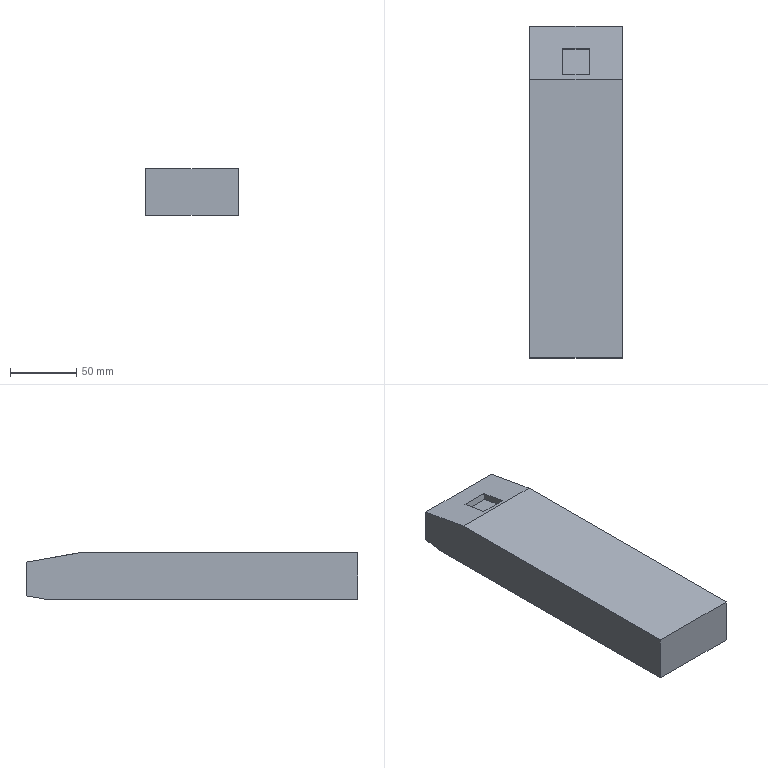Part | STEP file | 1 solid | 13 faces | box 70 x 250 x 35 mm | volume 599290 mm3 | plane 13
STEP:
#1=CARTESIAN_POINT('',(0.,0.,0.));
#2=DIRECTION('',(0.,0.,1.));
#3=DIRECTION('',(1.,0.,0.));
#4=AXIS2_PLACEMENT_3D('',#1,#2,#3);
#5=CARTESIAN_POINT('',(-77.862,-165.,-78.92));
#6=VERTEX_POINT('',#5);
#7=CARTESIAN_POINT('',(-77.862,-165.,-113.92));
#8=VERTEX_POINT('',#7);
#9=CARTESIAN_POINT('',(-77.862,-165.,-78.92));
#10=DIRECTION('',(0.,0.,-1.));
#11=VECTOR('',#10,1.);
#12=LINE('',#9,#11);
#13=CARTESIAN_POINT('',(-77.862,-165.,-113.92));
#14=DIRECTION('',(0.,-1.,0.));
#15=DIRECTION('',(0.,0.,-1.));
#16=AXIS2_PLACEMENT_3D('',#13,#14,#15);
#17=PLANE('',#16);
#18=CARTESIAN_POINT('',(-35.,0.));
#19=DIRECTION('',(1.,0.));
#20=VECTOR('',#19,1.);
#21=LINE('',#18,#20);
#22=(GEOMETRIC_REPRESENTATION_CONTEXT(2)PARAMETRIC_REPRESENTATION_CONTEXT()REPRESENTATION_CONTEXT('',''));
#23=DEFINITIONAL_REPRESENTATION('',(#21),#22);
#24=PCURVE('',#17,#23);
#25=CARTESIAN_POINT('',(-77.862,-150.,-78.92));
#26=DIRECTION('',(1.,0.,0.));
#27=DIRECTION('',(0.,0.,-1.));
#28=AXIS2_PLACEMENT_3D('',#25,#26,#27);
#29=PLANE('',#28);
#30=CARTESIAN_POINT('',(0.,-15.));
#31=DIRECTION('',(1.,0.));
#32=VECTOR('',#31,1.);
#33=LINE('',#30,#32);
#34=(GEOMETRIC_REPRESENTATION_CONTEXT(2)PARAMETRIC_REPRESENTATION_CONTEXT()REPRESENTATION_CONTEXT('',''));
#35=DEFINITIONAL_REPRESENTATION('',(#33),#34);
#36=PCURVE('',#29,#35);
#37=SURFACE_CURVE('',#12,(#24,#36),.PCURVE_S1.);
#38=EDGE_CURVE('',#6,#8,#37,.T.);
#39=ORIENTED_EDGE('',*,*,#38,.T.);
#40=CARTESIAN_POINT('',(-7.863,-165.,-113.92));
#41=VERTEX_POINT('',#40);
#42=CARTESIAN_POINT('',(-77.862,-165.,-113.92));
#43=DIRECTION('',(1.,0.,0.));
#44=VECTOR('',#43,1.);
#45=LINE('',#42,#44);
#46=CARTESIAN_POINT('',(0.,0.));
#47=DIRECTION('',(0.,1.));
#48=VECTOR('',#47,1.);
#49=LINE('',#46,#48);
#50=(GEOMETRIC_REPRESENTATION_CONTEXT(2)PARAMETRIC_REPRESENTATION_CONTEXT()REPRESENTATION_CONTEXT('',''));
#51=DEFINITIONAL_REPRESENTATION('',(#49),#50);
#52=PCURVE('',#17,#51);
#53=CARTESIAN_POINT('',(-77.862,-150.,-113.92));
#54=DIRECTION('',(0.,0.,1.));
#55=DIRECTION('',(1.,0.,0.));
#56=AXIS2_PLACEMENT_3D('',#53,#54,#55);
#57=PLANE('',#56);
#58=CARTESIAN_POINT('',(0.,-15.));
#59=DIRECTION('',(1.,0.));
#60=VECTOR('',#59,1.);
#61=LINE('',#58,#60);
#62=(GEOMETRIC_REPRESENTATION_CONTEXT(2)PARAMETRIC_REPRESENTATION_CONTEXT()REPRESENTATION_CONTEXT('',''));
#63=DEFINITIONAL_REPRESENTATION('',(#61),#62);
#64=PCURVE('',#57,#63);
#65=SURFACE_CURVE('',#45,(#52,#64),.PCURVE_S1.);
#66=EDGE_CURVE('',#8,#41,#65,.T.);
#67=ORIENTED_EDGE('',*,*,#66,.T.);
#68=CARTESIAN_POINT('',(-7.863,-165.,-78.92));
#69=VERTEX_POINT('',#68);
#70=CARTESIAN_POINT('',(-7.863,-165.,-113.92));
#71=DIRECTION('',(0.,0.,1.));
#72=VECTOR('',#71,1.);
#73=LINE('',#70,#72);
#74=CARTESIAN_POINT('',(0.,70.));
#75=DIRECTION('',(-1.,0.));
#76=VECTOR('',#75,1.);
#77=LINE('',#74,#76);
#78=(GEOMETRIC_REPRESENTATION_CONTEXT(2)PARAMETRIC_REPRESENTATION_CONTEXT()REPRESENTATION_CONTEXT('',''));
#79=DEFINITIONAL_REPRESENTATION('',(#77),#78);
#80=PCURVE('',#17,#79);
#81=CARTESIAN_POINT('',(-7.863,-150.,-113.92));
#82=DIRECTION('',(-1.,0.,0.));
#83=DIRECTION('',(0.,0.,1.));
#84=AXIS2_PLACEMENT_3D('',#81,#82,#83);
#85=PLANE('',#84);
#86=CARTESIAN_POINT('',(0.,-15.));
#87=DIRECTION('',(1.,0.));
#88=VECTOR('',#87,1.);
#89=LINE('',#86,#88);
#90=(GEOMETRIC_REPRESENTATION_CONTEXT(2)PARAMETRIC_REPRESENTATION_CONTEXT()REPRESENTATION_CONTEXT('',''));
#91=DEFINITIONAL_REPRESENTATION('',(#89),#90);
#92=PCURVE('',#85,#91);
#93=SURFACE_CURVE('',#73,(#80,#92),.PCURVE_S1.);
#94=EDGE_CURVE('',#41,#69,#93,.T.);
#95=ORIENTED_EDGE('',*,*,#94,.T.);
#96=CARTESIAN_POINT('',(-7.863,-165.,-78.92));
#97=DIRECTION('',(-1.,0.,0.));
#98=VECTOR('',#97,1.);
#99=LINE('',#96,#98);
#100=CARTESIAN_POINT('',(-35.,70.));
#101=DIRECTION('',(0.,-1.));
#102=VECTOR('',#101,1.);
#103=LINE('',#100,#102);
#104=(GEOMETRIC_REPRESENTATION_CONTEXT(2)PARAMETRIC_REPRESENTATION_CONTEXT()REPRESENTATION_CONTEXT('',''));
#105=DEFINITIONAL_REPRESENTATION('',(#103),#104);
#106=PCURVE('',#17,#105);
#107=CARTESIAN_POINT('',(-7.863,-150.,-78.92));
#108=DIRECTION('',(0.,0.,-1.));
#109=DIRECTION('',(-1.,0.,0.));
#110=AXIS2_PLACEMENT_3D('',#107,#108,#109);
#111=PLANE('',#110);
#112=CARTESIAN_POINT('',(0.,-15.));
#113=DIRECTION('',(1.,0.));
#114=VECTOR('',#113,1.);
#115=LINE('',#112,#114);
#116=(GEOMETRIC_REPRESENTATION_CONTEXT(2)PARAMETRIC_REPRESENTATION_CONTEXT()REPRESENTATION_CONTEXT('',''));
#117=DEFINITIONAL_REPRESENTATION('',(#115),#116);
#118=PCURVE('',#111,#117);
#119=SURFACE_CURVE('',#99,(#106,#118),.PCURVE_S1.);
#120=EDGE_CURVE('',#69,#6,#119,.T.);
#121=ORIENTED_EDGE('',*,*,#120,.T.);
#122=EDGE_LOOP('',(#39,#67,#95,#121));
#123=FACE_BOUND('',#122,.T.);
#124=ADVANCED_FACE('',(#123),#17,.T.);
#125=CARTESIAN_POINT('',(-7.863,45.,-78.92));
#126=VERTEX_POINT('',#125);
#127=CARTESIAN_POINT('',(-7.863,-150.,-78.92));
#128=DIRECTION('',(0.,1.,0.));
#129=VECTOR('',#128,1.);
#130=LINE('',#127,#129);
#131=CARTESIAN_POINT('',(0.,0.));
#132=DIRECTION('',(0.,1.));
#133=VECTOR('',#132,1.);
#134=LINE('',#131,#133);
#135=(GEOMETRIC_REPRESENTATION_CONTEXT(2)PARAMETRIC_REPRESENTATION_CONTEXT()REPRESENTATION_CONTEXT('',''));
#136=DEFINITIONAL_REPRESENTATION('',(#134),#135);
#137=PCURVE('',#111,#136);
#138=CARTESIAN_POINT('',(35.,0.));
#139=DIRECTION('',(0.,1.));
#140=VECTOR('',#139,1.);
#141=LINE('',#138,#140);
#142=(GEOMETRIC_REPRESENTATION_CONTEXT(2)PARAMETRIC_REPRESENTATION_CONTEXT()REPRESENTATION_CONTEXT('',''));
#143=DEFINITIONAL_REPRESENTATION('',(#141),#142);
#144=PCURVE('',#85,#143);
#145=SURFACE_CURVE('',#130,(#137,#144),.PCURVE_S1.);
#146=EDGE_CURVE('',#69,#126,#145,.T.);
#147=ORIENTED_EDGE('',*,*,#146,.T.);
#148=CARTESIAN_POINT('',(-77.862,45.,-78.92));
#149=VERTEX_POINT('',#148);
#150=CARTESIAN_POINT('',(-7.863,45.,-78.92));
#151=DIRECTION('',(-1.,0.,0.));
#152=VECTOR('',#151,1.);
#153=LINE('',#150,#152);
#154=CARTESIAN_POINT('',(0.,195.));
#155=DIRECTION('',(1.,0.));
#156=VECTOR('',#155,1.);
#157=LINE('',#154,#156);
#158=(GEOMETRIC_REPRESENTATION_CONTEXT(2)PARAMETRIC_REPRESENTATION_CONTEXT()REPRESENTATION_CONTEXT('',''));
#159=DEFINITIONAL_REPRESENTATION('',(#157),#158);
#160=PCURVE('',#111,#159);
#161=CARTESIAN_POINT('',(-7.863,45.,-78.92));
#162=DIRECTION('',(0.,0.1736,0.9848));
#163=DIRECTION('',(0.,-0.9848,0.1736));
#164=AXIS2_PLACEMENT_3D('',#161,#162,#163);
#165=PLANE('',#164);
#166=CARTESIAN_POINT('',(0.,0.));
#167=DIRECTION('',(0.,-1.));
#168=VECTOR('',#167,1.);
#169=LINE('',#166,#168);
#170=(GEOMETRIC_REPRESENTATION_CONTEXT(2)PARAMETRIC_REPRESENTATION_CONTEXT()REPRESENTATION_CONTEXT('',''));
#171=DEFINITIONAL_REPRESENTATION('',(#169),#170);
#172=PCURVE('',#165,#171);
#173=SURFACE_CURVE('',#153,(#160,#172),.PCURVE_S1.);
#174=EDGE_CURVE('',#126,#149,#173,.T.);
#175=ORIENTED_EDGE('',*,*,#174,.T.);
#176=CARTESIAN_POINT('',(-77.862,-150.,-78.92));
#177=DIRECTION('',(0.,1.,0.));
#178=VECTOR('',#177,1.);
#179=LINE('',#176,#178);
#180=CARTESIAN_POINT('',(70.,0.));
#181=DIRECTION('',(0.,1.));
#182=VECTOR('',#181,1.);
#183=LINE('',#180,#182);
#184=(GEOMETRIC_REPRESENTATION_CONTEXT(2)PARAMETRIC_REPRESENTATION_CONTEXT()REPRESENTATION_CONTEXT('',''));
#185=DEFINITIONAL_REPRESENTATION('',(#183),#184);
#186=PCURVE('',#111,#185);
#187=CARTESIAN_POINT('',(0.,0.));
#188=DIRECTION('',(0.,1.));
#189=VECTOR('',#188,1.);
#190=LINE('',#187,#189);
#191=(GEOMETRIC_REPRESENTATION_CONTEXT(2)PARAMETRIC_REPRESENTATION_CONTEXT()REPRESENTATION_CONTEXT('',''));
#192=DEFINITIONAL_REPRESENTATION('',(#190),#191);
#193=PCURVE('',#29,#192);
#194=SURFACE_CURVE('',#179,(#186,#193),.PCURVE_S1.);
#195=EDGE_CURVE('',#6,#149,#194,.T.);
#196=ORIENTED_EDGE('',*,*,#195,.F.);
#197=ORIENTED_EDGE('',*,*,#120,.F.);
#198=EDGE_LOOP('',(#147,#175,#196,#197));
#199=FACE_BOUND('',#198,.T.);
#200=ADVANCED_FACE('',(#199),#111,.F.);
#201=CARTESIAN_POINT('',(-7.863,70.5,-113.92));
#202=VERTEX_POINT('',#201);
#203=CARTESIAN_POINT('',(-7.863,-150.,-113.92));
#204=DIRECTION('',(0.,1.,0.));
#205=VECTOR('',#204,1.);
#206=LINE('',#203,#205);
#207=CARTESIAN_POINT('',(0.,0.));
#208=DIRECTION('',(0.,1.));
#209=VECTOR('',#208,1.);
#210=LINE('',#207,#209);
#211=(GEOMETRIC_REPRESENTATION_CONTEXT(2)PARAMETRIC_REPRESENTATION_CONTEXT()REPRESENTATION_CONTEXT('',''));
#212=DEFINITIONAL_REPRESENTATION('',(#210),#211);
#213=PCURVE('',#85,#212);
#214=CARTESIAN_POINT('',(70.,0.));
#215=DIRECTION('',(0.,1.));
#216=VECTOR('',#215,1.);
#217=LINE('',#214,#216);
#218=(GEOMETRIC_REPRESENTATION_CONTEXT(2)PARAMETRIC_REPRESENTATION_CONTEXT()REPRESENTATION_CONTEXT('',''));
#219=DEFINITIONAL_REPRESENTATION('',(#217),#218);
#220=PCURVE('',#57,#219);
#221=SURFACE_CURVE('',#206,(#213,#220),.PCURVE_S1.);
#222=EDGE_CURVE('',#41,#202,#221,.T.);
#223=ORIENTED_EDGE('',*,*,#222,.T.);
#224=CARTESIAN_POINT('',(-7.863,85.,-111.363));
#225=VERTEX_POINT('',#224);
#226=CARTESIAN_POINT('',(-7.863,-143.351,-151.627));
#227=DIRECTION('',(0.,0.9848,0.1736));
#228=VECTOR('',#227,1.);
#229=LINE('',#226,#228);
#230=CARTESIAN_POINT('',(-37.708,6.649));
#231=DIRECTION('',(0.1736,0.9848));
#232=VECTOR('',#231,1.);
#233=LINE('',#230,#232);
#234=(GEOMETRIC_REPRESENTATION_CONTEXT(2)PARAMETRIC_REPRESENTATION_CONTEXT()REPRESENTATION_CONTEXT('',''));
#235=DEFINITIONAL_REPRESENTATION('',(#233),#234);
#236=PCURVE('',#85,#235);
#237=CARTESIAN_POINT('',(-7.863,70.5,-113.92));
#238=DIRECTION('',(0.,0.1736,-0.9848));
#239=DIRECTION('',(0.,0.9848,0.1736));
#240=AXIS2_PLACEMENT_3D('',#237,#238,#239);
#241=PLANE('',#240);
#242=CARTESIAN_POINT('',(-217.15,0.));
#243=DIRECTION('',(1.,0.));
#244=VECTOR('',#243,1.);
#245=LINE('',#242,#244);
#246=(GEOMETRIC_REPRESENTATION_CONTEXT(2)PARAMETRIC_REPRESENTATION_CONTEXT()REPRESENTATION_CONTEXT('',''));
#247=DEFINITIONAL_REPRESENTATION('',(#245),#246);
#248=PCURVE('',#241,#247);
#249=SURFACE_CURVE('',#229,(#236,#248),.PCURVE_S1.);
#250=EDGE_CURVE('',#202,#225,#249,.T.);
#251=ORIENTED_EDGE('',*,*,#250,.T.);
#252=CARTESIAN_POINT('',(-7.863,85.,-85.973));
#253=VERTEX_POINT('',#252);
#254=CARTESIAN_POINT('',(-7.863,85.,-113.92));
#255=DIRECTION('',(0.,0.,1.));
#256=VECTOR('',#255,1.);
#257=LINE('',#254,#256);
#258=CARTESIAN_POINT('',(0.,235.));
#259=DIRECTION('',(1.,0.));
#260=VECTOR('',#259,1.);
#261=LINE('',#258,#260);
#262=(GEOMETRIC_REPRESENTATION_CONTEXT(2)PARAMETRIC_REPRESENTATION_CONTEXT()REPRESENTATION_CONTEXT('',''));
#263=DEFINITIONAL_REPRESENTATION('',(#261),#262);
#264=PCURVE('',#85,#263);
#265=CARTESIAN_POINT('',(-72.862,85.,-363.47));
#266=DIRECTION('',(0.,-1.,0.));
#267=DIRECTION('',(0.,0.,-1.));
#268=AXIS2_PLACEMENT_3D('',#265,#266,#267);
#269=PLANE('',#268);
#270=CARTESIAN_POINT('',(-249.551,65.));
#271=DIRECTION('',(-1.,0.));
#272=VECTOR('',#271,1.);
#273=LINE('',#270,#272);
#274=(GEOMETRIC_REPRESENTATION_CONTEXT(2)PARAMETRIC_REPRESENTATION_CONTEXT()REPRESENTATION_CONTEXT('',''));
#275=DEFINITIONAL_REPRESENTATION('',(#273),#274);
#276=PCURVE('',#269,#275);
#277=SURFACE_CURVE('',#257,(#264,#276),.PCURVE_S1.);
#278=EDGE_CURVE('',#225,#253,#277,.T.);
#279=ORIENTED_EDGE('',*,*,#278,.T.);
#280=CARTESIAN_POINT('',(-7.863,45.,-78.92));
#281=DIRECTION('',(0.,0.9848,-0.1736));
#282=VECTOR('',#281,1.);
#283=LINE('',#280,#282);
#284=CARTESIAN_POINT('',(35.,195.));
#285=DIRECTION('',(-0.1736,0.9848));
#286=VECTOR('',#285,1.);
#287=LINE('',#284,#286);
#288=(GEOMETRIC_REPRESENTATION_CONTEXT(2)PARAMETRIC_REPRESENTATION_CONTEXT()REPRESENTATION_CONTEXT('',''));
#289=DEFINITIONAL_REPRESENTATION('',(#287),#288);
#290=PCURVE('',#85,#289);
#291=CARTESIAN_POINT('',(0.,0.));
#292=DIRECTION('',(-1.,0.));
#293=VECTOR('',#292,1.);
#294=LINE('',#291,#293);
#295=(GEOMETRIC_REPRESENTATION_CONTEXT(2)PARAMETRIC_REPRESENTATION_CONTEXT()REPRESENTATION_CONTEXT('',''));
#296=DEFINITIONAL_REPRESENTATION('',(#294),#295);
#297=PCURVE('',#165,#296);
#298=SURFACE_CURVE('',#283,(#290,#297),.PCURVE_S1.);
#299=EDGE_CURVE('',#126,#253,#298,.T.);
#300=ORIENTED_EDGE('',*,*,#299,.F.);
#301=ORIENTED_EDGE('',*,*,#146,.F.);
#302=ORIENTED_EDGE('',*,*,#94,.F.);
#303=EDGE_LOOP('',(#223,#251,#279,#300,#301,#302));
#304=FACE_BOUND('',#303,.T.);
#305=ADVANCED_FACE('',(#304),#85,.F.);
#306=CARTESIAN_POINT('',(-77.862,70.5,-113.92));
#307=VERTEX_POINT('',#306);
#308=CARTESIAN_POINT('',(-77.862,-150.,-113.92));
#309=DIRECTION('',(0.,1.,0.));
#310=VECTOR('',#309,1.);
#311=LINE('',#308,#310);
#312=CARTESIAN_POINT('',(0.,0.));
#313=DIRECTION('',(0.,1.));
#314=VECTOR('',#313,1.);
#315=LINE('',#312,#314);
#316=(GEOMETRIC_REPRESENTATION_CONTEXT(2)PARAMETRIC_REPRESENTATION_CONTEXT()REPRESENTATION_CONTEXT('',''));
#317=DEFINITIONAL_REPRESENTATION('',(#315),#316);
#318=PCURVE('',#57,#317);
#319=CARTESIAN_POINT('',(35.,0.));
#320=DIRECTION('',(0.,1.));
#321=VECTOR('',#320,1.);
#322=LINE('',#319,#321);
#323=(GEOMETRIC_REPRESENTATION_CONTEXT(2)PARAMETRIC_REPRESENTATION_CONTEXT()REPRESENTATION_CONTEXT('',''));
#324=DEFINITIONAL_REPRESENTATION('',(#322),#323);
#325=PCURVE('',#29,#324);
#326=SURFACE_CURVE('',#311,(#318,#325),.PCURVE_S1.);
#327=EDGE_CURVE('',#8,#307,#326,.T.);
#328=ORIENTED_EDGE('',*,*,#327,.T.);
#329=CARTESIAN_POINT('',(-77.862,70.5,-113.92));
#330=DIRECTION('',(-1.,0.,0.));
#331=VECTOR('',#330,1.);
#332=LINE('',#329,#331);
#333=CARTESIAN_POINT('',(0.,220.5));
#334=DIRECTION('',(-1.,0.));
#335=VECTOR('',#334,1.);
#336=LINE('',#333,#335);
#337=(GEOMETRIC_REPRESENTATION_CONTEXT(2)PARAMETRIC_REPRESENTATION_CONTEXT()REPRESENTATION_CONTEXT('',''));
#338=DEFINITIONAL_REPRESENTATION('',(#336),#337);
#339=PCURVE('',#57,#338);
#340=CARTESIAN_POINT('',(0.,-70.));
#341=DIRECTION('',(0.,-1.));
#342=VECTOR('',#341,1.);
#343=LINE('',#340,#342);
#344=(GEOMETRIC_REPRESENTATION_CONTEXT(2)PARAMETRIC_REPRESENTATION_CONTEXT()REPRESENTATION_CONTEXT('',''));
#345=DEFINITIONAL_REPRESENTATION('',(#343),#344);
#346=PCURVE('',#241,#345);
#347=SURFACE_CURVE('',#332,(#339,#346),.PCURVE_S1.);
#348=EDGE_CURVE('',#202,#307,#347,.T.);
#349=ORIENTED_EDGE('',*,*,#348,.F.);
#350=ORIENTED_EDGE('',*,*,#222,.F.);
#351=ORIENTED_EDGE('',*,*,#66,.F.);
#352=EDGE_LOOP('',(#328,#349,#350,#351));
#353=FACE_BOUND('',#352,.T.);
#354=ADVANCED_FACE('',(#353),#57,.F.);
#355=ORIENTED_EDGE('',*,*,#195,.T.);
#356=CARTESIAN_POINT('',(-77.862,85.,-85.973));
#357=VERTEX_POINT('',#356);
#358=CARTESIAN_POINT('',(-77.862,-144.12,-45.573));
#359=DIRECTION('',(0.,0.9848,-0.1736));
#360=VECTOR('',#359,1.);
#361=LINE('',#358,#360);
#362=CARTESIAN_POINT('',(-33.347,5.88));
#363=DIRECTION('',(0.1736,0.9848));
#364=VECTOR('',#363,1.);
#365=LINE('',#362,#364);
#366=(GEOMETRIC_REPRESENTATION_CONTEXT(2)PARAMETRIC_REPRESENTATION_CONTEXT()REPRESENTATION_CONTEXT('',''));
#367=DEFINITIONAL_REPRESENTATION('',(#365),#366);
#368=PCURVE('',#29,#367);
#369=CARTESIAN_POINT('',(192.038,-70.));
#370=DIRECTION('',(-1.,0.));
#371=VECTOR('',#370,1.);
#372=LINE('',#369,#371);
#373=(GEOMETRIC_REPRESENTATION_CONTEXT(2)PARAMETRIC_REPRESENTATION_CONTEXT()REPRESENTATION_CONTEXT('',''));
#374=DEFINITIONAL_REPRESENTATION('',(#372),#373);
#375=PCURVE('',#165,#374);
#376=SURFACE_CURVE('',#361,(#368,#375),.PCURVE_S1.);
#377=EDGE_CURVE('',#149,#357,#376,.T.);
#378=ORIENTED_EDGE('',*,*,#377,.T.);
#379=CARTESIAN_POINT('',(-77.862,85.,-111.363));
#380=VERTEX_POINT('',#379);
#381=CARTESIAN_POINT('',(-77.862,85.,-78.92));
#382=DIRECTION('',(0.,0.,-1.));
#383=VECTOR('',#382,1.);
#384=LINE('',#381,#383);
#385=CARTESIAN_POINT('',(0.,235.));
#386=DIRECTION('',(1.,0.));
#387=VECTOR('',#386,1.);
#388=LINE('',#385,#387);
#389=(GEOMETRIC_REPRESENTATION_CONTEXT(2)PARAMETRIC_REPRESENTATION_CONTEXT()REPRESENTATION_CONTEXT('',''));
#390=DEFINITIONAL_REPRESENTATION('',(#388),#389);
#391=PCURVE('',#29,#390);
#392=CARTESIAN_POINT('',(-284.551,-5.));
#393=DIRECTION('',(1.,0.));
#394=VECTOR('',#393,1.);
#395=LINE('',#392,#394);
#396=(GEOMETRIC_REPRESENTATION_CONTEXT(2)PARAMETRIC_REPRESENTATION_CONTEXT()REPRESENTATION_CONTEXT('',''));
#397=DEFINITIONAL_REPRESENTATION('',(#395),#396);
#398=PCURVE('',#269,#397);
#399=SURFACE_CURVE('',#384,(#391,#398),.PCURVE_S1.);
#400=EDGE_CURVE('',#357,#380,#399,.T.);
#401=ORIENTED_EDGE('',*,*,#400,.T.);
#402=CARTESIAN_POINT('',(-77.862,70.5,-113.92));
#403=DIRECTION('',(0.,0.9848,0.1736));
#404=VECTOR('',#403,1.);
#405=LINE('',#402,#404);
#406=CARTESIAN_POINT('',(35.,220.5));
#407=DIRECTION('',(-0.1736,0.9848));
#408=VECTOR('',#407,1.);
#409=LINE('',#406,#408);
#410=(GEOMETRIC_REPRESENTATION_CONTEXT(2)PARAMETRIC_REPRESENTATION_CONTEXT()REPRESENTATION_CONTEXT('',''));
#411=DEFINITIONAL_REPRESENTATION('',(#409),#410);
#412=PCURVE('',#29,#411);
#413=CARTESIAN_POINT('',(0.,-70.));
#414=DIRECTION('',(1.,0.));
#415=VECTOR('',#414,1.);
#416=LINE('',#413,#415);
#417=(GEOMETRIC_REPRESENTATION_CONTEXT(2)PARAMETRIC_REPRESENTATION_CONTEXT()REPRESENTATION_CONTEXT('',''));
#418=DEFINITIONAL_REPRESENTATION('',(#416),#417);
#419=PCURVE('',#241,#418);
#420=SURFACE_CURVE('',#405,(#412,#419),.PCURVE_S1.);
#421=EDGE_CURVE('',#307,#380,#420,.T.);
#422=ORIENTED_EDGE('',*,*,#421,.F.);
#423=ORIENTED_EDGE('',*,*,#327,.F.);
#424=ORIENTED_EDGE('',*,*,#38,.F.);
#425=EDGE_LOOP('',(#355,#378,#401,#422,#423,#424));
#426=FACE_BOUND('',#425,.T.);
#427=ADVANCED_FACE('',(#426),#29,.F.);
#428=CARTESIAN_POINT('',(-52.862,48.188,-79.482));
#429=VERTEX_POINT('',#428);
#430=CARTESIAN_POINT('',(-32.862,48.188,-79.482));
#431=VERTEX_POINT('',#430);
#432=CARTESIAN_POINT('',(-7.863,48.188,-79.482));
#433=DIRECTION('',(1.,0.,0.));
#434=VECTOR('',#433,1.);
#435=LINE('',#432,#434);
#436=CARTESIAN_POINT('',(-3.237,0.));
#437=DIRECTION('',(0.,1.));
#438=VECTOR('',#437,1.);
#439=LINE('',#436,#438);
#440=(GEOMETRIC_REPRESENTATION_CONTEXT(2)PARAMETRIC_REPRESENTATION_CONTEXT()REPRESENTATION_CONTEXT('',''));
#441=DEFINITIONAL_REPRESENTATION('',(#439),#440);
#442=PCURVE('',#165,#441);
#443=CARTESIAN_POINT('',(-43.112,49.924,-69.634));
#444=DIRECTION('',(0.,-0.9848,0.1736));
#445=DIRECTION('',(0.,-0.1736,-0.9848));
#446=AXIS2_PLACEMENT_3D('',#443,#444,#445);
#447=PLANE('',#446);
#448=CARTESIAN_POINT('',(10.,35.25));
#449=DIRECTION('',(0.,1.));
#450=VECTOR('',#449,1.);
#451=LINE('',#448,#450);
#452=(GEOMETRIC_REPRESENTATION_CONTEXT(2)PARAMETRIC_REPRESENTATION_CONTEXT()REPRESENTATION_CONTEXT('',''));
#453=DEFINITIONAL_REPRESENTATION('',(#451),#452);
#454=PCURVE('',#447,#453);
#455=SURFACE_CURVE('',#435,(#442,#454),.PCURVE_S1.);
#456=EDGE_CURVE('',#429,#431,#455,.T.);
#457=ORIENTED_EDGE('',*,*,#456,.F.);
#458=CARTESIAN_POINT('',(-52.862,68.264,-83.022));
#459=VERTEX_POINT('',#458);
#460=CARTESIAN_POINT('',(-52.862,45.,-78.92));
#461=DIRECTION('',(0.,0.9848,-0.1736));
#462=VECTOR('',#461,1.);
#463=LINE('',#460,#462);
#464=CARTESIAN_POINT('',(0.,-45.));
#465=DIRECTION('',(-1.,0.));
#466=VECTOR('',#465,1.);
#467=LINE('',#464,#466);
#468=(GEOMETRIC_REPRESENTATION_CONTEXT(2)PARAMETRIC_REPRESENTATION_CONTEXT()REPRESENTATION_CONTEXT('',''));
#469=DEFINITIONAL_REPRESENTATION('',(#467),#468);
#470=PCURVE('',#165,#469);
#471=CARTESIAN_POINT('',(-52.862,0.,-92.47));
#472=DIRECTION('',(-1.,0.,0.));
#473=DIRECTION('',(0.,0.,1.));
#474=AXIS2_PLACEMENT_3D('',#471,#472,#473);
#475=PLANE('',#474);
#476=CARTESIAN_POINT('',(13.551,45.));
#477=DIRECTION('',(-0.1736,0.9848));
#478=VECTOR('',#477,1.);
#479=LINE('',#476,#478);
#480=(GEOMETRIC_REPRESENTATION_CONTEXT(2)PARAMETRIC_REPRESENTATION_CONTEXT()REPRESENTATION_CONTEXT('',''));
#481=DEFINITIONAL_REPRESENTATION('',(#479),#480);
#482=PCURVE('',#475,#481);
#483=SURFACE_CURVE('',#463,(#470,#482),.PCURVE_S1.);
#484=EDGE_CURVE('',#429,#459,#483,.T.);
#485=ORIENTED_EDGE('',*,*,#484,.T.);
#486=CARTESIAN_POINT('',(-32.862,68.264,-83.022));
#487=VERTEX_POINT('',#486);
#488=CARTESIAN_POINT('',(-7.863,68.264,-83.022));
#489=DIRECTION('',(1.,0.,0.));
#490=VECTOR('',#489,1.);
#491=LINE('',#488,#490);
#492=CARTESIAN_POINT('',(-23.622,0.));
#493=DIRECTION('',(0.,1.));
#494=VECTOR('',#493,1.);
#495=LINE('',#492,#494);
#496=(GEOMETRIC_REPRESENTATION_CONTEXT(2)PARAMETRIC_REPRESENTATION_CONTEXT()REPRESENTATION_CONTEXT('',''));
#497=DEFINITIONAL_REPRESENTATION('',(#495),#496);
#498=PCURVE('',#165,#497);
#499=CARTESIAN_POINT('',(-43.112,70.,-73.173));
#500=DIRECTION('',(0.,0.9848,-0.1736));
#501=DIRECTION('',(0.,0.1736,0.9848));
#502=AXIS2_PLACEMENT_3D('',#499,#500,#501);
#503=PLANE('',#502);
#504=CARTESIAN_POINT('',(-10.,35.25));
#505=DIRECTION('',(0.,1.));
#506=VECTOR('',#505,1.);
#507=LINE('',#504,#506);
#508=(GEOMETRIC_REPRESENTATION_CONTEXT(2)PARAMETRIC_REPRESENTATION_CONTEXT()REPRESENTATION_CONTEXT('',''));
#509=DEFINITIONAL_REPRESENTATION('',(#507),#508);
#510=PCURVE('',#503,#509);
#511=SURFACE_CURVE('',#491,(#498,#510),.PCURVE_S1.);
#512=EDGE_CURVE('',#459,#487,#511,.T.);
#513=ORIENTED_EDGE('',*,*,#512,.T.);
#514=CARTESIAN_POINT('',(-32.862,45.,-78.92));
#515=DIRECTION('',(0.,-0.9848,0.1736));
#516=VECTOR('',#515,1.);
#517=LINE('',#514,#516);
#518=CARTESIAN_POINT('',(0.,-25.));
#519=DIRECTION('',(1.,0.));
#520=VECTOR('',#519,1.);
#521=LINE('',#518,#520);
#522=(GEOMETRIC_REPRESENTATION_CONTEXT(2)PARAMETRIC_REPRESENTATION_CONTEXT()REPRESENTATION_CONTEXT('',''));
#523=DEFINITIONAL_REPRESENTATION('',(#521),#522);
#524=PCURVE('',#165,#523);
#525=CARTESIAN_POINT('',(-32.862,0.,-92.47));
#526=DIRECTION('',(1.,0.,0.));
#527=DIRECTION('',(0.,0.,-1.));
#528=AXIS2_PLACEMENT_3D('',#525,#526,#527);
#529=PLANE('',#528);
#530=CARTESIAN_POINT('',(-13.551,45.));
#531=DIRECTION('',(-0.1736,-0.9848));
#532=VECTOR('',#531,1.);
#533=LINE('',#530,#532);
#534=(GEOMETRIC_REPRESENTATION_CONTEXT(2)PARAMETRIC_REPRESENTATION_CONTEXT()REPRESENTATION_CONTEXT('',''));
#535=DEFINITIONAL_REPRESENTATION('',(#533),#534);
#536=PCURVE('',#529,#535);
#537=SURFACE_CURVE('',#517,(#524,#536),.PCURVE_S1.);
#538=EDGE_CURVE('',#487,#431,#537,.T.);
#539=ORIENTED_EDGE('',*,*,#538,.T.);
#540=EDGE_LOOP('',(#457,#485,#513,#539));
#541=FACE_BOUND('',#540,.T.);
#542=ORIENTED_EDGE('',*,*,#299,.T.);
#543=CARTESIAN_POINT('',(-7.863,85.,-85.973));
#544=DIRECTION('',(-1.,0.,0.));
#545=VECTOR('',#544,1.);
#546=LINE('',#543,#545);
#547=CARTESIAN_POINT('',(-40.617,0.));
#548=DIRECTION('',(0.,-1.));
#549=VECTOR('',#548,1.);
#550=LINE('',#547,#549);
#551=(GEOMETRIC_REPRESENTATION_CONTEXT(2)PARAMETRIC_REPRESENTATION_CONTEXT()REPRESENTATION_CONTEXT('',''));
#552=DEFINITIONAL_REPRESENTATION('',(#550),#551);
#553=PCURVE('',#165,#552);
#554=CARTESIAN_POINT('',(-277.498,65.));
#555=DIRECTION('',(0.,-1.));
#556=VECTOR('',#555,1.);
#557=LINE('',#554,#556);
#558=(GEOMETRIC_REPRESENTATION_CONTEXT(2)PARAMETRIC_REPRESENTATION_CONTEXT()REPRESENTATION_CONTEXT('',''));
#559=DEFINITIONAL_REPRESENTATION('',(#557),#558);
#560=PCURVE('',#269,#559);
#561=SURFACE_CURVE('',#546,(#553,#560),.PCURVE_S1.);
#562=EDGE_CURVE('',#253,#357,#561,.T.);
#563=ORIENTED_EDGE('',*,*,#562,.T.);
#564=ORIENTED_EDGE('',*,*,#377,.F.);
#565=ORIENTED_EDGE('',*,*,#174,.F.);
#566=EDGE_LOOP('',(#542,#563,#564,#565));
#567=FACE_BOUND('',#566,.T.);
#568=ADVANCED_FACE('',(#541,#567),#165,.T.);
#569=ORIENTED_EDGE('',*,*,#400,.F.);
#570=ORIENTED_EDGE('',*,*,#562,.F.);
#571=ORIENTED_EDGE('',*,*,#278,.F.);
#572=CARTESIAN_POINT('',(-7.863,85.,-111.363));
#573=DIRECTION('',(1.,0.,0.));
#574=VECTOR('',#573,1.);
#575=LINE('',#572,#574);
#576=CARTESIAN_POINT('',(-252.107,65.));
#577=DIRECTION('',(0.,1.));
#578=VECTOR('',#577,1.);
#579=LINE('',#576,#578);
#580=(GEOMETRIC_REPRESENTATION_CONTEXT(2)PARAMETRIC_REPRESENTATION_CONTEXT()REPRESENTATION_CONTEXT('',''));
#581=DEFINITIONAL_REPRESENTATION('',(#579),#580);
#582=PCURVE('',#269,#581);
#583=CARTESIAN_POINT('',(14.724,0.));
#584=DIRECTION('',(0.,1.));
#585=VECTOR('',#584,1.);
#586=LINE('',#583,#585);
#587=(GEOMETRIC_REPRESENTATION_CONTEXT(2)PARAMETRIC_REPRESENTATION_CONTEXT()REPRESENTATION_CONTEXT('',''));
#588=DEFINITIONAL_REPRESENTATION('',(#586),#587);
#589=PCURVE('',#241,#588);
#590=SURFACE_CURVE('',#575,(#582,#589),.PCURVE_S1.);
#591=EDGE_CURVE('',#380,#225,#590,.T.);
#592=ORIENTED_EDGE('',*,*,#591,.F.);
#593=EDGE_LOOP('',(#569,#570,#571,#592));
#594=FACE_BOUND('',#593,.T.);
#595=ADVANCED_FACE('',(#594),#269,.F.);
#596=ORIENTED_EDGE('',*,*,#250,.F.);
#597=ORIENTED_EDGE('',*,*,#348,.T.);
#598=ORIENTED_EDGE('',*,*,#421,.T.);
#599=ORIENTED_EDGE('',*,*,#591,.T.);
#600=EDGE_LOOP('',(#596,#597,#598,#599));
#601=FACE_BOUND('',#600,.T.);
#602=ADVANCED_FACE('',(#601),#241,.T.);
#603=CARTESIAN_POINT('',(-52.862,67.395,-87.946));
#604=VERTEX_POINT('',#603);
#605=CARTESIAN_POINT('',(-52.862,70.,-73.173));
#606=DIRECTION('',(0.,0.1736,0.9848));
#607=VECTOR('',#606,1.);
#608=LINE('',#605,#607);
#609=CARTESIAN_POINT('',(0.,-9.75));
#610=DIRECTION('',(1.,0.));
#611=VECTOR('',#610,1.);
#612=LINE('',#609,#611);
#613=(GEOMETRIC_REPRESENTATION_CONTEXT(2)PARAMETRIC_REPRESENTATION_CONTEXT()REPRESENTATION_CONTEXT('',''));
#614=DEFINITIONAL_REPRESENTATION('',(#612),#613);
#615=PCURVE('',#503,#614);
#616=CARTESIAN_POINT('',(19.297,70.));
#617=DIRECTION('',(0.9848,0.1736));
#618=VECTOR('',#617,1.);
#619=LINE('',#616,#618);
#620=(GEOMETRIC_REPRESENTATION_CONTEXT(2)PARAMETRIC_REPRESENTATION_CONTEXT()REPRESENTATION_CONTEXT('',''));
#621=DEFINITIONAL_REPRESENTATION('',(#619),#620);
#622=PCURVE('',#475,#621);
#623=SURFACE_CURVE('',#608,(#615,#622),.PCURVE_S1.);
#624=EDGE_CURVE('',#604,#459,#623,.T.);
#625=ORIENTED_EDGE('',*,*,#624,.F.);
#626=CARTESIAN_POINT('',(-32.862,67.395,-87.946));
#627=VERTEX_POINT('',#626);
#628=CARTESIAN_POINT('',(-43.112,67.395,-87.946));
#629=DIRECTION('',(-1.,0.,0.));
#630=VECTOR('',#629,1.);
#631=LINE('',#628,#630);
#632=CARTESIAN_POINT('',(-15.,0.));
#633=DIRECTION('',(0.,-1.));
#634=VECTOR('',#633,1.);
#635=LINE('',#632,#634);
#636=(GEOMETRIC_REPRESENTATION_CONTEXT(2)PARAMETRIC_REPRESENTATION_CONTEXT()REPRESENTATION_CONTEXT('',''));
#637=DEFINITIONAL_REPRESENTATION('',(#635),#636);
#638=PCURVE('',#503,#637);
#639=CARTESIAN_POINT('',(-7.863,44.132,-83.844));
#640=DIRECTION('',(0.,0.1736,0.9848));
#641=DIRECTION('',(0.,-0.9848,0.1736));
#642=AXIS2_PLACEMENT_3D('',#639,#640,#641);
#643=PLANE('',#642);
#644=CARTESIAN_POINT('',(-23.622,-35.25));
#645=DIRECTION('',(0.,-1.));
#646=VECTOR('',#645,1.);
#647=LINE('',#644,#646);
#648=(GEOMETRIC_REPRESENTATION_CONTEXT(2)PARAMETRIC_REPRESENTATION_CONTEXT()REPRESENTATION_CONTEXT('',''));
#649=DEFINITIONAL_REPRESENTATION('',(#647),#648);
#650=PCURVE('',#643,#649);
#651=SURFACE_CURVE('',#631,(#638,#650),.PCURVE_S1.);
#652=EDGE_CURVE('',#627,#604,#651,.T.);
#653=ORIENTED_EDGE('',*,*,#652,.F.);
#654=CARTESIAN_POINT('',(-32.862,64.589,-103.859));
#655=DIRECTION('',(0.,0.1736,0.9848));
#656=VECTOR('',#655,1.);
#657=LINE('',#654,#656);
#658=CARTESIAN_POINT('',(-31.159,10.25));
#659=DIRECTION('',(1.,0.));
#660=VECTOR('',#659,1.);
#661=LINE('',#658,#660);
#662=(GEOMETRIC_REPRESENTATION_CONTEXT(2)PARAMETRIC_REPRESENTATION_CONTEXT()REPRESENTATION_CONTEXT('',''));
#663=DEFINITIONAL_REPRESENTATION('',(#661),#662);
#664=PCURVE('',#503,#663);
#665=CARTESIAN_POINT('',(11.389,64.589));
#666=DIRECTION('',(-0.9848,0.1736));
#667=VECTOR('',#666,1.);
#668=LINE('',#665,#667);
#669=(GEOMETRIC_REPRESENTATION_CONTEXT(2)PARAMETRIC_REPRESENTATION_CONTEXT()REPRESENTATION_CONTEXT('',''));
#670=DEFINITIONAL_REPRESENTATION('',(#668),#669);
#671=PCURVE('',#529,#670);
#672=SURFACE_CURVE('',#657,(#664,#671),.PCURVE_S1.);
#673=EDGE_CURVE('',#627,#487,#672,.T.);
#674=ORIENTED_EDGE('',*,*,#673,.T.);
#675=ORIENTED_EDGE('',*,*,#512,.F.);
#676=EDGE_LOOP('',(#625,#653,#674,#675));
#677=FACE_BOUND('',#676,.T.);
#678=ADVANCED_FACE('',(#677),#503,.F.);
#679=ORIENTED_EDGE('',*,*,#456,.T.);
#680=CARTESIAN_POINT('',(-32.862,47.319,-84.406));
#681=VERTEX_POINT('',#680);
#682=CARTESIAN_POINT('',(-32.862,44.513,-100.319));
#683=DIRECTION('',(0.,0.1736,0.9848));
#684=VECTOR('',#683,1.);
#685=LINE('',#682,#684);
#686=CARTESIAN_POINT('',(31.159,10.25));
#687=DIRECTION('',(-1.,0.));
#688=VECTOR('',#687,1.);
#689=LINE('',#686,#688);
#690=(GEOMETRIC_REPRESENTATION_CONTEXT(2)PARAMETRIC_REPRESENTATION_CONTEXT()REPRESENTATION_CONTEXT('',''));
#691=DEFINITIONAL_REPRESENTATION('',(#689),#690);
#692=PCURVE('',#447,#691);
#693=CARTESIAN_POINT('',(7.849,44.513));
#694=DIRECTION('',(-0.9848,0.1736));
#695=VECTOR('',#694,1.);
#696=LINE('',#693,#695);
#697=(GEOMETRIC_REPRESENTATION_CONTEXT(2)PARAMETRIC_REPRESENTATION_CONTEXT()REPRESENTATION_CONTEXT('',''));
#698=DEFINITIONAL_REPRESENTATION('',(#696),#697);
#699=PCURVE('',#529,#698);
#700=SURFACE_CURVE('',#685,(#692,#699),.PCURVE_S1.);
#701=EDGE_CURVE('',#681,#431,#700,.T.);
#702=ORIENTED_EDGE('',*,*,#701,.F.);
#703=CARTESIAN_POINT('',(-52.862,47.319,-84.406));
#704=VERTEX_POINT('',#703);
#705=CARTESIAN_POINT('',(-43.112,47.319,-84.406));
#706=DIRECTION('',(-1.,0.,0.));
#707=VECTOR('',#706,1.);
#708=LINE('',#705,#707);
#709=CARTESIAN_POINT('',(15.,0.));
#710=DIRECTION('',(0.,-1.));
#711=VECTOR('',#710,1.);
#712=LINE('',#709,#711);
#713=(GEOMETRIC_REPRESENTATION_CONTEXT(2)PARAMETRIC_REPRESENTATION_CONTEXT()REPRESENTATION_CONTEXT('',''));
#714=DEFINITIONAL_REPRESENTATION('',(#712),#713);
#715=PCURVE('',#447,#714);
#716=CARTESIAN_POINT('',(-3.237,-35.25));
#717=DIRECTION('',(0.,-1.));
#718=VECTOR('',#717,1.);
#719=LINE('',#716,#718);
#720=(GEOMETRIC_REPRESENTATION_CONTEXT(2)PARAMETRIC_REPRESENTATION_CONTEXT()REPRESENTATION_CONTEXT('',''));
#721=DEFINITIONAL_REPRESENTATION('',(#719),#720);
#722=PCURVE('',#643,#721);
#723=SURFACE_CURVE('',#708,(#715,#722),.PCURVE_S1.);
#724=EDGE_CURVE('',#681,#704,#723,.T.);
#725=ORIENTED_EDGE('',*,*,#724,.T.);
#726=CARTESIAN_POINT('',(-52.862,44.513,-100.319));
#727=DIRECTION('',(0.,-0.1736,-0.9848));
#728=VECTOR('',#727,1.);
#729=LINE('',#726,#728);
#730=CARTESIAN_POINT('',(31.159,-9.75));
#731=DIRECTION('',(1.,0.));
#732=VECTOR('',#731,1.);
#733=LINE('',#730,#732);
#734=(GEOMETRIC_REPRESENTATION_CONTEXT(2)PARAMETRIC_REPRESENTATION_CONTEXT()REPRESENTATION_CONTEXT('',''));
#735=DEFINITIONAL_REPRESENTATION('',(#733),#734);
#736=PCURVE('',#447,#735);
#737=CARTESIAN_POINT('',(-7.849,44.513));
#738=DIRECTION('',(-0.9848,-0.1736));
#739=VECTOR('',#738,1.);
#740=LINE('',#737,#739);
#741=(GEOMETRIC_REPRESENTATION_CONTEXT(2)PARAMETRIC_REPRESENTATION_CONTEXT()REPRESENTATION_CONTEXT('',''));
#742=DEFINITIONAL_REPRESENTATION('',(#740),#741);
#743=PCURVE('',#475,#742);
#744=SURFACE_CURVE('',#729,(#736,#743),.PCURVE_S1.);
#745=EDGE_CURVE('',#429,#704,#744,.T.);
#746=ORIENTED_EDGE('',*,*,#745,.F.);
#747=EDGE_LOOP('',(#679,#702,#725,#746));
#748=FACE_BOUND('',#747,.T.);
#749=ADVANCED_FACE('',(#748),#447,.F.);
#750=ORIENTED_EDGE('',*,*,#745,.T.);
#751=CARTESIAN_POINT('',(-52.862,2.806,-76.557));
#752=DIRECTION('',(0.,-0.9848,0.1736));
#753=VECTOR('',#752,1.);
#754=LINE('',#751,#753);
#755=CARTESIAN_POINT('',(15.914,2.806));
#756=DIRECTION('',(0.1736,-0.9848));
#757=VECTOR('',#756,1.);
#758=LINE('',#755,#757);
#759=(GEOMETRIC_REPRESENTATION_CONTEXT(2)PARAMETRIC_REPRESENTATION_CONTEXT()REPRESENTATION_CONTEXT('',''));
#760=DEFINITIONAL_REPRESENTATION('',(#758),#759);
#761=PCURVE('',#475,#760);
#762=CARTESIAN_POINT('',(41.963,-45.));
#763=DIRECTION('',(1.,0.));
#764=VECTOR('',#763,1.);
#765=LINE('',#762,#764);
#766=(GEOMETRIC_REPRESENTATION_CONTEXT(2)PARAMETRIC_REPRESENTATION_CONTEXT()REPRESENTATION_CONTEXT('',''));
#767=DEFINITIONAL_REPRESENTATION('',(#765),#766);
#768=PCURVE('',#643,#767);
#769=SURFACE_CURVE('',#754,(#761,#768),.PCURVE_S1.);
#770=EDGE_CURVE('',#604,#704,#769,.T.);
#771=ORIENTED_EDGE('',*,*,#770,.F.);
#772=ORIENTED_EDGE('',*,*,#624,.T.);
#773=ORIENTED_EDGE('',*,*,#484,.F.);
#774=EDGE_LOOP('',(#750,#771,#772,#773));
#775=FACE_BOUND('',#774,.T.);
#776=ADVANCED_FACE('',(#775),#475,.F.);
#777=ORIENTED_EDGE('',*,*,#673,.F.);
#778=CARTESIAN_POINT('',(-32.862,2.806,-76.557));
#779=DIRECTION('',(0.,0.9848,-0.1736));
#780=VECTOR('',#779,1.);
#781=LINE('',#778,#780);
#782=CARTESIAN_POINT('',(-15.914,2.806));
#783=DIRECTION('',(0.1736,0.9848));
#784=VECTOR('',#783,1.);
#785=LINE('',#782,#784);
#786=(GEOMETRIC_REPRESENTATION_CONTEXT(2)PARAMETRIC_REPRESENTATION_CONTEXT()REPRESENTATION_CONTEXT('',''));
#787=DEFINITIONAL_REPRESENTATION('',(#785),#786);
#788=PCURVE('',#529,#787);
#789=CARTESIAN_POINT('',(41.963,-25.));
#790=DIRECTION('',(-1.,0.));
#791=VECTOR('',#790,1.);
#792=LINE('',#789,#791);
#793=(GEOMETRIC_REPRESENTATION_CONTEXT(2)PARAMETRIC_REPRESENTATION_CONTEXT()REPRESENTATION_CONTEXT('',''));
#794=DEFINITIONAL_REPRESENTATION('',(#792),#793);
#795=PCURVE('',#643,#794);
#796=SURFACE_CURVE('',#781,(#788,#795),.PCURVE_S1.);
#797=EDGE_CURVE('',#681,#627,#796,.T.);
#798=ORIENTED_EDGE('',*,*,#797,.F.);
#799=ORIENTED_EDGE('',*,*,#701,.T.);
#800=ORIENTED_EDGE('',*,*,#538,.F.);
#801=EDGE_LOOP('',(#777,#798,#799,#800));
#802=FACE_BOUND('',#801,.T.);
#803=ADVANCED_FACE('',(#802),#529,.F.);
#804=ORIENTED_EDGE('',*,*,#724,.F.);
#805=ORIENTED_EDGE('',*,*,#797,.T.);
#806=ORIENTED_EDGE('',*,*,#652,.T.);
#807=ORIENTED_EDGE('',*,*,#770,.T.);
#808=EDGE_LOOP('',(#804,#805,#806,#807));
#809=FACE_BOUND('',#808,.T.);
#810=ADVANCED_FACE('',(#809),#643,.T.);
#811=CLOSED_SHELL('',(#124,#200,#305,#354,#427,#568,#595,#602,#678,#749,#776,#803,#810));
#812=MANIFOLD_SOLID_BREP('',#811);
#813=(LENGTH_UNIT()NAMED_UNIT(*)SI_UNIT(.MILLI.,.METRE.));
#814=UNCERTAINTY_MEASURE_WITH_UNIT(LENGTH_MEASURE(0.0000001),#813,'','');
#815=(NAMED_UNIT(*)PLANE_ANGLE_UNIT()SI_UNIT($,.RADIAN.));
#816=(NAMED_UNIT(*)SI_UNIT($,.STERADIAN.)SOLID_ANGLE_UNIT());
#817=(GEOMETRIC_REPRESENTATION_CONTEXT(3)GLOBAL_UNCERTAINTY_ASSIGNED_CONTEXT((#814))GLOBAL_UNIT_ASSIGNED_CONTEXT((#813,#815,#816))REPRESENTATION_CONTEXT('',''));
#818=ADVANCED_BREP_SHAPE_REPRESENTATION('',(#4,#812),#817);